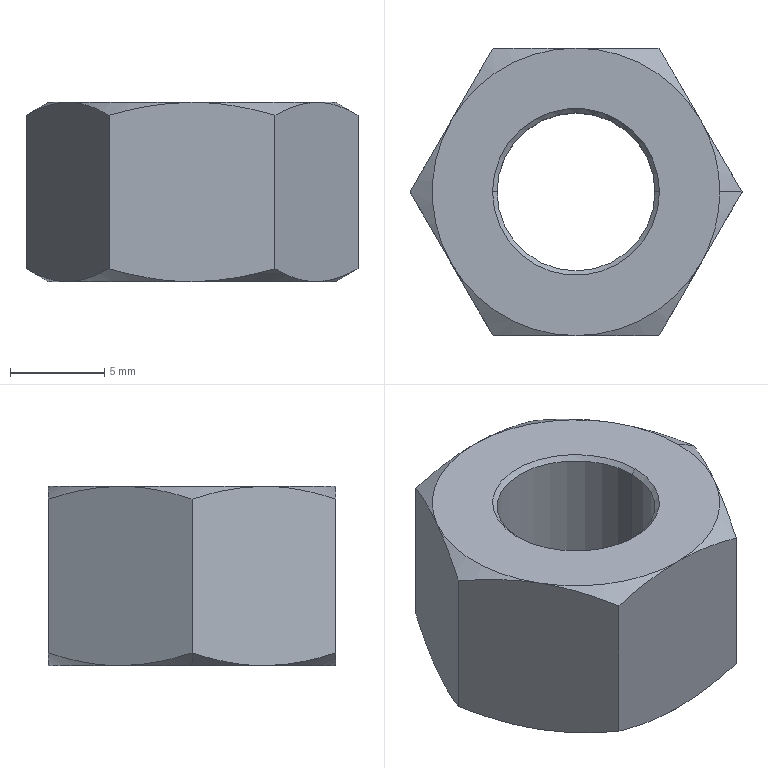Part | SolidWorks | features Cut 2, Chamfer 1, Extrusion 1 | 1 solid | 28 faces | box 17.6 x 15.242 x 9.5 mm | volume 1379 mm3 | cone 18 | plane 8 | cylinder 2 | commonest cylinder face diameters 8.376 x2
STEP:
#1=CARTESIAN_POINT('',(-4.188,0.,9.262));
#2=VERTEX_POINT('',#1);
#3=CARTESIAN_POINT('',(4.188,0.,9.262));
#4=VERTEX_POINT('',#3);
#5=CARTESIAN_POINT('',(0.,0.,9.262));
#6=DIRECTION('',(0.,0.,1.));
#7=DIRECTION('',(-1.,0.,0.));
#8=AXIS2_PLACEMENT_3D('',#5,#6,#7);
#9=CIRCLE('',#8,4.188);
#10=EDGE_CURVE('',#2,#4,#9,.T.);
#11=ORIENTED_EDGE('',*,*,#10,.F.);
#12=CARTESIAN_POINT('',(-4.426,0.,9.5));
#13=VERTEX_POINT('',#12);
#14=CARTESIAN_POINT('',(-4.188,0.,9.262));
#15=DIRECTION('',(-0.7071,0.,0.7071));
#16=VECTOR('',#15,1000.);
#17=LINE('',#14,#16);
#18=EDGE_CURVE('',#2,#13,#17,.T.);
#19=ORIENTED_EDGE('',*,*,#18,.T.);
#20=CARTESIAN_POINT('',(4.426,0.,9.5));
#21=VERTEX_POINT('',#20);
#22=CARTESIAN_POINT('',(0.,0.,9.5));
#23=DIRECTION('',(0.,0.,-1.));
#24=DIRECTION('',(-1.,0.,0.));
#25=AXIS2_PLACEMENT_3D('',#22,#23,#24);
#26=CIRCLE('',#25,4.426);
#27=EDGE_CURVE('',#21,#13,#26,.T.);
#28=ORIENTED_EDGE('',*,*,#27,.F.);
#29=CARTESIAN_POINT('',(4.188,0.,9.262));
#30=DIRECTION('',(0.7071,0.,0.7071));
#31=VECTOR('',#30,1000.);
#32=LINE('',#29,#31);
#33=EDGE_CURVE('',#4,#21,#32,.T.);
#34=ORIENTED_EDGE('',*,*,#33,.F.);
#35=EDGE_LOOP('',(#11,#19,#28,#34));
#36=FACE_OUTER_BOUND('',#35,.T.);
#37=CARTESIAN_POINT('',(0.,0.,9.262));
#38=DIRECTION('',(0.,0.,1.));
#39=DIRECTION('',(1.,0.,0.));
#40=AXIS2_PLACEMENT_3D('',#37,#38,#39);
#41=CONICAL_SURFACE('',#40,4.188,0.7854);
#42=ADVANCED_FACE('',(#36),#41,.F.);
#43=CARTESIAN_POINT('',(4.188,0.,0.2375));
#44=VERTEX_POINT('',#43);
#45=CARTESIAN_POINT('',(-4.188,0.,0.2375));
#46=VERTEX_POINT('',#45);
#47=CARTESIAN_POINT('',(0.,0.,0.2375));
#48=DIRECTION('',(0.,0.,-1.));
#49=DIRECTION('',(-1.,0.,0.));
#50=AXIS2_PLACEMENT_3D('',#47,#48,#49);
#51=CIRCLE('',#50,4.188);
#52=EDGE_CURVE('',#44,#46,#51,.T.);
#53=ORIENTED_EDGE('',*,*,#52,.F.);
#54=CARTESIAN_POINT('',(4.426,0.,0.));
#55=VERTEX_POINT('',#54);
#56=CARTESIAN_POINT('',(4.426,0.,0.));
#57=DIRECTION('',(0.7071,0.,-0.7071));
#58=VECTOR('',#57,1000.);
#59=LINE('',#56,#58);
#60=EDGE_CURVE('',#44,#55,#59,.T.);
#61=ORIENTED_EDGE('',*,*,#60,.T.);
#62=CARTESIAN_POINT('',(-4.426,0.,0.));
#63=VERTEX_POINT('',#62);
#64=CARTESIAN_POINT('',(0.,0.,0.));
#65=DIRECTION('',(0.,0.,1.));
#66=DIRECTION('',(-1.,0.,0.));
#67=AXIS2_PLACEMENT_3D('',#64,#65,#66);
#68=CIRCLE('',#67,4.426);
#69=EDGE_CURVE('',#63,#55,#68,.T.);
#70=ORIENTED_EDGE('',*,*,#69,.F.);
#71=CARTESIAN_POINT('',(-4.426,0.,0.));
#72=DIRECTION('',(-0.7071,0.,-0.7071));
#73=VECTOR('',#72,1000.);
#74=LINE('',#71,#73);
#75=EDGE_CURVE('',#46,#63,#74,.T.);
#76=ORIENTED_EDGE('',*,*,#75,.F.);
#77=EDGE_LOOP('',(#53,#61,#70,#76));
#78=FACE_OUTER_BOUND('',#77,.T.);
#79=CARTESIAN_POINT('',(0.,0.,0.));
#80=DIRECTION('',(0.,0.,-1.));
#81=DIRECTION('',(-1.,0.,0.));
#82=AXIS2_PLACEMENT_3D('',#79,#80,#81);
#83=CONICAL_SURFACE('',#82,4.426,0.7854);
#84=ADVANCED_FACE('',(#78),#83,.F.);
#85=CARTESIAN_POINT('',(6.6,3.811,9.5));
#86=VERTEX_POINT('',#85);
#87=CARTESIAN_POINT('',(7.621,0.,9.5));
#88=VERTEX_POINT('',#87);
#89=CARTESIAN_POINT('',(0.,0.,9.5));
#90=DIRECTION('',(0.,0.,-1.));
#91=DIRECTION('',(-1.,0.,0.));
#92=AXIS2_PLACEMENT_3D('',#89,#90,#91);
#93=CIRCLE('',#92,7.621);
#94=EDGE_CURVE('',#86,#88,#93,.T.);
#95=ORIENTED_EDGE('',*,*,#94,.T.);
#96=CARTESIAN_POINT('',(8.8,0.,8.819));
#97=VERTEX_POINT('',#96);
#98=CARTESIAN_POINT('',(7.621,0.,9.5));
#99=DIRECTION('',(0.866,0.,-0.5));
#100=VECTOR('',#99,1000.);
#101=LINE('',#98,#100);
#102=EDGE_CURVE('',#88,#97,#101,.T.);
#103=ORIENTED_EDGE('',*,*,#102,.T.);
#104=CARTESIAN_POINT('',(8.8,0.,8.819));
#105=CARTESIAN_POINT('',(8.44,0.6233,9.027));
#106=CARTESIAN_POINT('',(8.078,1.251,9.198));
#107=CARTESIAN_POINT('',(7.345,2.52,9.435));
#108=CARTESIAN_POINT('',(6.975,3.161,9.5));
#109=CARTESIAN_POINT('',(6.6,3.811,9.5));
#110=B_SPLINE_CURVE_WITH_KNOTS('',3,(#104,#105,#106,#107,#108,#109),.UNSPECIFIED.,.F.,.F.,(4,2,4),(0.000000238,0.002226,0.004452),.UNSPECIFIED.);
#111=EDGE_CURVE('',#97,#86,#110,.T.);
#112=ORIENTED_EDGE('',*,*,#111,.T.);
#113=EDGE_LOOP('',(#95,#103,#112));
#114=FACE_OUTER_BOUND('',#113,.T.);
#115=CARTESIAN_POINT('',(0.,0.,9.5));
#116=DIRECTION('',(0.,0.,-1.));
#117=DIRECTION('',(1.,0.,0.));
#118=AXIS2_PLACEMENT_3D('',#115,#116,#117);
#119=CONICAL_SURFACE('',#118,7.621,1.047);
#120=ADVANCED_FACE('',(#114),#119,.T.);
#121=CARTESIAN_POINT('',(-7.621,0.,0.));
#122=VERTEX_POINT('',#121);
#123=CARTESIAN_POINT('',(-6.6,3.811,0.));
#124=VERTEX_POINT('',#123);
#125=CARTESIAN_POINT('',(0.,0.,0.));
#126=DIRECTION('',(0.,0.,-1.));
#127=DIRECTION('',(-1.,0.,0.));
#128=AXIS2_PLACEMENT_3D('',#125,#126,#127);
#129=CIRCLE('',#128,7.621);
#130=EDGE_CURVE('',#122,#124,#129,.T.);
#131=ORIENTED_EDGE('',*,*,#130,.F.);
#132=CARTESIAN_POINT('',(-8.8,0.,0.6807));
#133=VERTEX_POINT('',#132);
#134=CARTESIAN_POINT('',(-7.621,0.,0.));
#135=DIRECTION('',(-0.866,0.,0.5));
#136=VECTOR('',#135,1000.);
#137=LINE('',#134,#136);
#138=EDGE_CURVE('',#122,#133,#137,.T.);
#139=ORIENTED_EDGE('',*,*,#138,.T.);
#140=CARTESIAN_POINT('',(-8.8,0.,0.6807));
#141=CARTESIAN_POINT('',(-8.44,0.6233,0.4729));
#142=CARTESIAN_POINT('',(-8.078,1.251,0.3017));
#143=CARTESIAN_POINT('',(-7.345,2.52,0.06487));
#144=CARTESIAN_POINT('',(-6.975,3.161,0.));
#145=CARTESIAN_POINT('',(-6.6,3.811,0.));
#146=B_SPLINE_CURVE_WITH_KNOTS('',3,(#140,#141,#142,#143,#144,#145),.UNSPECIFIED.,.F.,.F.,(4,2,4),(0.000000238,0.002226,0.004452),.UNSPECIFIED.);
#147=EDGE_CURVE('',#133,#124,#146,.T.);
#148=ORIENTED_EDGE('',*,*,#147,.T.);
#149=EDGE_LOOP('',(#131,#139,#148));
#150=FACE_OUTER_BOUND('',#149,.T.);
#151=CARTESIAN_POINT('',(0.,0.,0.));
#152=DIRECTION('',(0.,0.,1.));
#153=DIRECTION('',(-1.,0.,0.));
#154=AXIS2_PLACEMENT_3D('',#151,#152,#153);
#155=CONICAL_SURFACE('',#154,7.621,1.047);
#156=ADVANCED_FACE('',(#150),#155,.T.);
#157=ORIENTED_EDGE('',*,*,#10,.T.);
#158=CARTESIAN_POINT('',(4.188,0.,9.5));
#159=DIRECTION('',(0.,0.,-1.));
#160=VECTOR('',#159,1000.);
#161=LINE('',#158,#160);
#162=EDGE_CURVE('',#4,#44,#161,.T.);
#163=ORIENTED_EDGE('',*,*,#162,.T.);
#164=ORIENTED_EDGE('',*,*,#52,.T.);
#165=CARTESIAN_POINT('',(-4.188,0.,9.5));
#166=DIRECTION('',(0.,0.,-1.));
#167=VECTOR('',#166,1000.);
#168=LINE('',#165,#167);
#169=EDGE_CURVE('',#2,#46,#168,.T.);
#170=ORIENTED_EDGE('',*,*,#169,.F.);
#171=EDGE_LOOP('',(#157,#163,#164,#170));
#172=FACE_OUTER_BOUND('',#171,.T.);
#173=CARTESIAN_POINT('',(0.,0.,9.5));
#174=DIRECTION('',(0.,0.,-1.));
#175=DIRECTION('',(-1.,0.,0.));
#176=AXIS2_PLACEMENT_3D('',#173,#174,#175);
#177=CYLINDRICAL_SURFACE('',#176,4.188);
#178=ADVANCED_FACE('',(#172),#177,.F.);
#179=ORIENTED_EDGE('',*,*,#111,.F.);
#180=CARTESIAN_POINT('',(8.8,0.,0.6807));
#181=VERTEX_POINT('',#180);
#182=CARTESIAN_POINT('',(8.8,0.,9.5));
#183=DIRECTION('',(0.,0.,-1.));
#184=VECTOR('',#183,1000.);
#185=LINE('',#182,#184);
#186=EDGE_CURVE('',#97,#181,#185,.T.);
#187=ORIENTED_EDGE('',*,*,#186,.T.);
#188=CARTESIAN_POINT('',(6.6,3.811,0.));
#189=VERTEX_POINT('',#188);
#190=CARTESIAN_POINT('',(6.6,3.811,0.));
#191=CARTESIAN_POINT('',(6.787,3.487,0.));
#192=CARTESIAN_POINT('',(6.974,3.162,0.01609));
#193=CARTESIAN_POINT('',(7.345,2.52,0.07835));
#194=CARTESIAN_POINT('',(7.53,2.201,0.1245));
#195=CARTESIAN_POINT('',(8.079,1.249,0.3023));
#196=CARTESIAN_POINT('',(8.441,0.6218,0.4734));
#197=CARTESIAN_POINT('',(8.8,0.,0.6807));
#198=B_SPLINE_CURVE_WITH_KNOTS('',3,(#190,#191,#192,#193,#194,#195,#196,#197),.UNSPECIFIED.,.F.,.F.,(4,2,2,4),(0.004452,0.005561,0.00667,0.008888),.UNSPECIFIED.);
#199=EDGE_CURVE('',#189,#181,#198,.T.);
#200=ORIENTED_EDGE('',*,*,#199,.F.);
#201=CARTESIAN_POINT('',(4.4,7.621,0.6807));
#202=VERTEX_POINT('',#201);
#203=CARTESIAN_POINT('',(4.4,7.621,0.6807));
#204=CARTESIAN_POINT('',(4.76,6.998,0.4729));
#205=CARTESIAN_POINT('',(5.122,6.37,0.3017));
#206=CARTESIAN_POINT('',(5.855,5.101,0.06487));
#207=CARTESIAN_POINT('',(6.225,4.46,0.));
#208=CARTESIAN_POINT('',(6.6,3.811,0.));
#209=B_SPLINE_CURVE_WITH_KNOTS('',3,(#203,#204,#205,#206,#207,#208),.UNSPECIFIED.,.F.,.F.,(4,2,4),(0.000000238,0.002226,0.004452),.UNSPECIFIED.);
#210=EDGE_CURVE('',#202,#189,#209,.T.);
#211=ORIENTED_EDGE('',*,*,#210,.F.);
#212=CARTESIAN_POINT('',(4.4,7.621,8.819));
#213=VERTEX_POINT('',#212);
#214=CARTESIAN_POINT('',(4.4,7.621,9.5));
#215=DIRECTION('',(0.,0.,-1.));
#216=VECTOR('',#215,1000.);
#217=LINE('',#214,#216);
#218=EDGE_CURVE('',#213,#202,#217,.T.);
#219=ORIENTED_EDGE('',*,*,#218,.F.);
#220=CARTESIAN_POINT('',(6.6,3.811,9.5));
#221=CARTESIAN_POINT('',(6.413,4.134,9.5));
#222=CARTESIAN_POINT('',(6.226,4.459,9.484));
#223=CARTESIAN_POINT('',(5.855,5.101,9.422));
#224=CARTESIAN_POINT('',(5.67,5.42,9.376));
#225=CARTESIAN_POINT('',(5.121,6.372,9.198));
#226=CARTESIAN_POINT('',(4.759,6.999,9.027));
#227=CARTESIAN_POINT('',(4.4,7.621,8.819));
#228=B_SPLINE_CURVE_WITH_KNOTS('',3,(#220,#221,#222,#223,#224,#225,#226,#227),.UNSPECIFIED.,.F.,.F.,(4,2,2,4),(0.004452,0.005561,0.00667,0.008888),.UNSPECIFIED.);
#229=EDGE_CURVE('',#86,#213,#228,.T.);
#230=ORIENTED_EDGE('',*,*,#229,.F.);
#231=EDGE_LOOP('',(#179,#187,#200,#211,#219,#230));
#232=FACE_OUTER_BOUND('',#231,.T.);
#233=CARTESIAN_POINT('',(8.8,0.,9.5));
#234=DIRECTION('',(-0.866,-0.5,0.));
#235=DIRECTION('',(0.5,-0.866,0.));
#236=AXIS2_PLACEMENT_3D('',#233,#234,#235);
#237=PLANE('',#236);
#238=ADVANCED_FACE('',(#232),#237,.F.);
#239=CARTESIAN_POINT('',(0.,7.621,9.5));
#240=VERTEX_POINT('',#239);
#241=CARTESIAN_POINT('',(4.4,7.621,8.819));
#242=CARTESIAN_POINT('',(3.688,7.621,9.025));
#243=CARTESIAN_POINT('',(2.968,7.621,9.196));
#244=CARTESIAN_POINT('',(1.499,7.621,9.434));
#245=CARTESIAN_POINT('',(0.7447,7.621,9.5));
#246=CARTESIAN_POINT('',(0.,7.621,9.5));
#247=B_SPLINE_CURVE_WITH_KNOTS('',3,(#241,#242,#243,#244,#245,#246),.UNSPECIFIED.,.F.,.F.,(4,2,4),(0.02521,0.02744,0.02967),.UNSPECIFIED.);
#248=EDGE_CURVE('',#213,#240,#247,.T.);
#249=ORIENTED_EDGE('',*,*,#248,.F.);
#250=ORIENTED_EDGE('',*,*,#218,.T.);
#251=CARTESIAN_POINT('',(0.,7.621,0.));
#252=VERTEX_POINT('',#251);
#253=CARTESIAN_POINT('',(0.,7.621,0.));
#254=CARTESIAN_POINT('',(0.7447,7.621,0.));
#255=CARTESIAN_POINT('',(1.499,7.621,0.06582));
#256=CARTESIAN_POINT('',(2.968,7.621,0.3043));
#257=CARTESIAN_POINT('',(3.688,7.621,0.4753));
#258=CARTESIAN_POINT('',(4.4,7.621,0.6807));
#259=B_SPLINE_CURVE_WITH_KNOTS('',3,(#253,#254,#255,#256,#257,#258),.UNSPECIFIED.,.F.,.F.,(4,2,4),(0.01252,0.01475,0.01698),.UNSPECIFIED.);
#260=EDGE_CURVE('',#252,#202,#259,.T.);
#261=ORIENTED_EDGE('',*,*,#260,.F.);
#262=CARTESIAN_POINT('',(-4.4,7.621,0.6807));
#263=VERTEX_POINT('',#262);
#264=CARTESIAN_POINT('',(-4.4,7.621,0.6807));
#265=CARTESIAN_POINT('',(-3.684,7.621,0.4739));
#266=CARTESIAN_POINT('',(-2.951,7.621,0.3008));
#267=CARTESIAN_POINT('',(-1.483,7.621,0.06401));
#268=CARTESIAN_POINT('',(-0.7442,7.621,0.));
#269=CARTESIAN_POINT('',(0.,7.621,0.));
#270=B_SPLINE_CURVE_WITH_KNOTS('',3,(#264,#265,#266,#267,#268,#269),.UNSPECIFIED.,.F.,.F.,(4,2,4),(0.008069,0.0103,0.01252),.UNSPECIFIED.);
#271=EDGE_CURVE('',#263,#252,#270,.T.);
#272=ORIENTED_EDGE('',*,*,#271,.F.);
#273=CARTESIAN_POINT('',(-4.4,7.621,8.819));
#274=VERTEX_POINT('',#273);
#275=CARTESIAN_POINT('',(-4.4,7.621,9.5));
#276=DIRECTION('',(0.,0.,-1.));
#277=VECTOR('',#276,1000.);
#278=LINE('',#275,#277);
#279=EDGE_CURVE('',#274,#263,#278,.T.);
#280=ORIENTED_EDGE('',*,*,#279,.F.);
#281=CARTESIAN_POINT('',(0.,7.621,9.5));
#282=CARTESIAN_POINT('',(-0.7442,7.621,9.5));
#283=CARTESIAN_POINT('',(-1.483,7.621,9.436));
#284=CARTESIAN_POINT('',(-2.951,7.621,9.199));
#285=CARTESIAN_POINT('',(-3.684,7.621,9.026));
#286=CARTESIAN_POINT('',(-4.4,7.621,8.819));
#287=B_SPLINE_CURVE_WITH_KNOTS('',3,(#281,#282,#283,#284,#285,#286),.UNSPECIFIED.,.F.,.F.,(4,2,4),(0.02967,0.0319,0.03412),.UNSPECIFIED.);
#288=EDGE_CURVE('',#240,#274,#287,.T.);
#289=ORIENTED_EDGE('',*,*,#288,.F.);
#290=EDGE_LOOP('',(#249,#250,#261,#272,#280,#289));
#291=FACE_OUTER_BOUND('',#290,.T.);
#292=CARTESIAN_POINT('',(4.4,7.621,9.5));
#293=DIRECTION('',(0.,-1.,0.));
#294=DIRECTION('',(1.,0.,0.));
#295=AXIS2_PLACEMENT_3D('',#292,#293,#294);
#296=PLANE('',#295);
#297=ADVANCED_FACE('',(#291),#296,.F.);
#298=CARTESIAN_POINT('',(-6.6,3.811,9.5));
#299=VERTEX_POINT('',#298);
#300=CARTESIAN_POINT('',(-4.4,7.621,8.819));
#301=CARTESIAN_POINT('',(-4.76,6.998,9.027));
#302=CARTESIAN_POINT('',(-5.122,6.37,9.198));
#303=CARTESIAN_POINT('',(-5.855,5.101,9.435));
#304=CARTESIAN_POINT('',(-6.225,4.46,9.5));
#305=CARTESIAN_POINT('',(-6.6,3.811,9.5));
#306=B_SPLINE_CURVE_WITH_KNOTS('',3,(#300,#301,#302,#303,#304,#305),.UNSPECIFIED.,.F.,.F.,(4,2,4),(0.000000238,0.002226,0.004452),.UNSPECIFIED.);
#307=EDGE_CURVE('',#274,#299,#306,.T.);
#308=ORIENTED_EDGE('',*,*,#307,.F.);
#309=ORIENTED_EDGE('',*,*,#279,.T.);
#310=CARTESIAN_POINT('',(-6.6,3.811,0.));
#311=CARTESIAN_POINT('',(-6.413,4.134,0.));
#312=CARTESIAN_POINT('',(-6.226,4.459,0.01609));
#313=CARTESIAN_POINT('',(-5.855,5.101,0.07835));
#314=CARTESIAN_POINT('',(-5.67,5.42,0.1245));
#315=CARTESIAN_POINT('',(-5.121,6.372,0.3023));
#316=CARTESIAN_POINT('',(-4.759,6.999,0.4734));
#317=CARTESIAN_POINT('',(-4.4,7.621,0.6807));
#318=B_SPLINE_CURVE_WITH_KNOTS('',3,(#310,#311,#312,#313,#314,#315,#316,#317),.UNSPECIFIED.,.F.,.F.,(4,2,2,4),(0.004452,0.005561,0.00667,0.008888),.UNSPECIFIED.);
#319=EDGE_CURVE('',#124,#263,#318,.T.);
#320=ORIENTED_EDGE('',*,*,#319,.F.);
#321=ORIENTED_EDGE('',*,*,#147,.F.);
#322=CARTESIAN_POINT('',(-8.8,0.,8.819));
#323=VERTEX_POINT('',#322);
#324=CARTESIAN_POINT('',(-8.8,0.,9.5));
#325=DIRECTION('',(0.,0.,-1.));
#326=VECTOR('',#325,1000.);
#327=LINE('',#324,#326);
#328=EDGE_CURVE('',#323,#133,#327,.T.);
#329=ORIENTED_EDGE('',*,*,#328,.F.);
#330=CARTESIAN_POINT('',(-6.6,3.811,9.5));
#331=CARTESIAN_POINT('',(-6.787,3.487,9.5));
#332=CARTESIAN_POINT('',(-6.974,3.162,9.484));
#333=CARTESIAN_POINT('',(-7.345,2.52,9.422));
#334=CARTESIAN_POINT('',(-7.53,2.201,9.376));
#335=CARTESIAN_POINT('',(-8.079,1.249,9.198));
#336=CARTESIAN_POINT('',(-8.441,0.6218,9.027));
#337=CARTESIAN_POINT('',(-8.8,0.,8.819));
#338=B_SPLINE_CURVE_WITH_KNOTS('',3,(#330,#331,#332,#333,#334,#335,#336,#337),.UNSPECIFIED.,.F.,.F.,(4,2,2,4),(0.004452,0.005561,0.00667,0.008888),.UNSPECIFIED.);
#339=EDGE_CURVE('',#299,#323,#338,.T.);
#340=ORIENTED_EDGE('',*,*,#339,.F.);
#341=EDGE_LOOP('',(#308,#309,#320,#321,#329,#340));
#342=FACE_OUTER_BOUND('',#341,.T.);
#343=CARTESIAN_POINT('',(-4.4,7.621,9.5));
#344=DIRECTION('',(0.866,-0.5,0.));
#345=DIRECTION('',(0.5,0.866,0.));
#346=AXIS2_PLACEMENT_3D('',#343,#344,#345);
#347=PLANE('',#346);
#348=ADVANCED_FACE('',(#342),#347,.F.);
#349=CARTESIAN_POINT('',(-6.6,-3.811,9.5));
#350=VERTEX_POINT('',#349);
#351=CARTESIAN_POINT('',(-8.8,0.,8.819));
#352=CARTESIAN_POINT('',(-8.44,-0.6233,9.027));
#353=CARTESIAN_POINT('',(-8.078,-1.251,9.198));
#354=CARTESIAN_POINT('',(-7.345,-2.52,9.435));
#355=CARTESIAN_POINT('',(-6.975,-3.161,9.5));
#356=CARTESIAN_POINT('',(-6.6,-3.811,9.5));
#357=B_SPLINE_CURVE_WITH_KNOTS('',3,(#351,#352,#353,#354,#355,#356),.UNSPECIFIED.,.F.,.F.,(4,2,4),(0.000000238,0.002226,0.004452),.UNSPECIFIED.);
#358=EDGE_CURVE('',#323,#350,#357,.T.);
#359=ORIENTED_EDGE('',*,*,#358,.F.);
#360=ORIENTED_EDGE('',*,*,#328,.T.);
#361=CARTESIAN_POINT('',(-6.6,-3.811,0.));
#362=VERTEX_POINT('',#361);
#363=CARTESIAN_POINT('',(-6.6,-3.811,0.));
#364=CARTESIAN_POINT('',(-6.787,-3.487,0.));
#365=CARTESIAN_POINT('',(-6.974,-3.162,0.01609));
#366=CARTESIAN_POINT('',(-7.345,-2.52,0.07835));
#367=CARTESIAN_POINT('',(-7.53,-2.201,0.1245));
#368=CARTESIAN_POINT('',(-8.079,-1.249,0.3023));
#369=CARTESIAN_POINT('',(-8.441,-0.6218,0.4734));
#370=CARTESIAN_POINT('',(-8.8,0.,0.6807));
#371=B_SPLINE_CURVE_WITH_KNOTS('',3,(#363,#364,#365,#366,#367,#368,#369,#370),.UNSPECIFIED.,.F.,.F.,(4,2,2,4),(0.004452,0.005561,0.00667,0.008888),.UNSPECIFIED.);
#372=EDGE_CURVE('',#362,#133,#371,.T.);
#373=ORIENTED_EDGE('',*,*,#372,.F.);
#374=CARTESIAN_POINT('',(-4.4,-7.621,0.6807));
#375=VERTEX_POINT('',#374);
#376=CARTESIAN_POINT('',(-4.4,-7.621,0.6807));
#377=CARTESIAN_POINT('',(-4.76,-6.998,0.4729));
#378=CARTESIAN_POINT('',(-5.122,-6.37,0.3017));
#379=CARTESIAN_POINT('',(-5.855,-5.101,0.06487));
#380=CARTESIAN_POINT('',(-6.225,-4.46,0.));
#381=CARTESIAN_POINT('',(-6.6,-3.811,0.));
#382=B_SPLINE_CURVE_WITH_KNOTS('',3,(#376,#377,#378,#379,#380,#381),.UNSPECIFIED.,.F.,.F.,(4,2,4),(0.000000238,0.002226,0.004452),.UNSPECIFIED.);
#383=EDGE_CURVE('',#375,#362,#382,.T.);
#384=ORIENTED_EDGE('',*,*,#383,.F.);
#385=CARTESIAN_POINT('',(-4.4,-7.621,8.819));
#386=VERTEX_POINT('',#385);
#387=CARTESIAN_POINT('',(-4.4,-7.621,9.5));
#388=DIRECTION('',(0.,0.,-1.));
#389=VECTOR('',#388,1000.);
#390=LINE('',#387,#389);
#391=EDGE_CURVE('',#386,#375,#390,.T.);
#392=ORIENTED_EDGE('',*,*,#391,.F.);
#393=CARTESIAN_POINT('',(-6.6,-3.811,9.5));
#394=CARTESIAN_POINT('',(-6.413,-4.134,9.5));
#395=CARTESIAN_POINT('',(-6.226,-4.459,9.484));
#396=CARTESIAN_POINT('',(-5.855,-5.101,9.422));
#397=CARTESIAN_POINT('',(-5.67,-5.42,9.376));
#398=CARTESIAN_POINT('',(-5.121,-6.372,9.198));
#399=CARTESIAN_POINT('',(-4.759,-6.999,9.027));
#400=CARTESIAN_POINT('',(-4.4,-7.621,8.819));
#401=B_SPLINE_CURVE_WITH_KNOTS('',3,(#393,#394,#395,#396,#397,#398,#399,#400),.UNSPECIFIED.,.F.,.F.,(4,2,2,4),(0.004452,0.005561,0.00667,0.008888),.UNSPECIFIED.);
#402=EDGE_CURVE('',#350,#386,#401,.T.);
#403=ORIENTED_EDGE('',*,*,#402,.F.);
#404=EDGE_LOOP('',(#359,#360,#373,#384,#392,#403));
#405=FACE_OUTER_BOUND('',#404,.T.);
#406=CARTESIAN_POINT('',(-8.8,0.,9.5));
#407=DIRECTION('',(0.866,0.5,0.));
#408=DIRECTION('',(-0.5,0.866,0.));
#409=AXIS2_PLACEMENT_3D('',#406,#407,#408);
#410=PLANE('',#409);
#411=ADVANCED_FACE('',(#405),#410,.F.);
#412=CARTESIAN_POINT('',(0.,-7.621,9.5));
#413=VERTEX_POINT('',#412);
#414=CARTESIAN_POINT('',(-4.4,-7.621,8.819));
#415=CARTESIAN_POINT('',(-3.684,-7.621,9.026));
#416=CARTESIAN_POINT('',(-2.951,-7.621,9.199));
#417=CARTESIAN_POINT('',(-1.483,-7.621,9.436));
#418=CARTESIAN_POINT('',(-0.7442,-7.621,9.5));
#419=CARTESIAN_POINT('',(0.,-7.621,9.5));
#420=B_SPLINE_CURVE_WITH_KNOTS('',3,(#414,#415,#416,#417,#418,#419),.UNSPECIFIED.,.F.,.F.,(4,2,4),(0.008069,0.0103,0.01252),.UNSPECIFIED.);
#421=EDGE_CURVE('',#386,#413,#420,.T.);
#422=ORIENTED_EDGE('',*,*,#421,.F.);
#423=ORIENTED_EDGE('',*,*,#391,.T.);
#424=CARTESIAN_POINT('',(0.,-7.621,0.));
#425=VERTEX_POINT('',#424);
#426=CARTESIAN_POINT('',(0.,-7.621,0.));
#427=CARTESIAN_POINT('',(-0.7442,-7.621,0.));
#428=CARTESIAN_POINT('',(-1.483,-7.621,0.06401));
#429=CARTESIAN_POINT('',(-2.951,-7.621,0.3008));
#430=CARTESIAN_POINT('',(-3.684,-7.621,0.4739));
#431=CARTESIAN_POINT('',(-4.4,-7.621,0.6807));
#432=B_SPLINE_CURVE_WITH_KNOTS('',3,(#426,#427,#428,#429,#430,#431),.UNSPECIFIED.,.F.,.F.,(4,2,4),(0.02967,0.0319,0.03412),.UNSPECIFIED.);
#433=EDGE_CURVE('',#425,#375,#432,.T.);
#434=ORIENTED_EDGE('',*,*,#433,.F.);
#435=CARTESIAN_POINT('',(4.4,-7.621,0.6807));
#436=VERTEX_POINT('',#435);
#437=CARTESIAN_POINT('',(4.4,-7.621,0.6807));
#438=CARTESIAN_POINT('',(3.688,-7.621,0.4753));
#439=CARTESIAN_POINT('',(2.968,-7.621,0.3043));
#440=CARTESIAN_POINT('',(1.499,-7.621,0.06582));
#441=CARTESIAN_POINT('',(0.7447,-7.621,0.));
#442=CARTESIAN_POINT('',(0.,-7.621,0.));
#443=B_SPLINE_CURVE_WITH_KNOTS('',3,(#437,#438,#439,#440,#441,#442),.UNSPECIFIED.,.F.,.F.,(4,2,4),(0.02521,0.02744,0.02967),.UNSPECIFIED.);
#444=EDGE_CURVE('',#436,#425,#443,.T.);
#445=ORIENTED_EDGE('',*,*,#444,.F.);
#446=CARTESIAN_POINT('',(4.4,-7.621,8.819));
#447=VERTEX_POINT('',#446);
#448=CARTESIAN_POINT('',(4.4,-7.621,9.5));
#449=DIRECTION('',(0.,0.,-1.));
#450=VECTOR('',#449,1000.);
#451=LINE('',#448,#450);
#452=EDGE_CURVE('',#447,#436,#451,.T.);
#453=ORIENTED_EDGE('',*,*,#452,.F.);
#454=CARTESIAN_POINT('',(0.,-7.621,9.5));
#455=CARTESIAN_POINT('',(0.7447,-7.621,9.5));
#456=CARTESIAN_POINT('',(1.499,-7.621,9.434));
#457=CARTESIAN_POINT('',(2.968,-7.621,9.196));
#458=CARTESIAN_POINT('',(3.688,-7.621,9.025));
#459=CARTESIAN_POINT('',(4.4,-7.621,8.819));
#460=B_SPLINE_CURVE_WITH_KNOTS('',3,(#454,#455,#456,#457,#458,#459),.UNSPECIFIED.,.F.,.F.,(4,2,4),(0.01252,0.01475,0.01698),.UNSPECIFIED.);
#461=EDGE_CURVE('',#413,#447,#460,.T.);
#462=ORIENTED_EDGE('',*,*,#461,.F.);
#463=EDGE_LOOP('',(#422,#423,#434,#445,#453,#462));
#464=FACE_OUTER_BOUND('',#463,.T.);
#465=CARTESIAN_POINT('',(-4.4,-7.621,9.5));
#466=DIRECTION('',(0.,1.,0.));
#467=DIRECTION('',(0.,0.,1.));
#468=AXIS2_PLACEMENT_3D('',#465,#466,#467);
#469=PLANE('',#468);
#470=ADVANCED_FACE('',(#464),#469,.F.);
#471=CARTESIAN_POINT('',(6.6,-3.811,9.5));
#472=VERTEX_POINT('',#471);
#473=CARTESIAN_POINT('',(4.4,-7.621,8.819));
#474=CARTESIAN_POINT('',(4.76,-6.998,9.027));
#475=CARTESIAN_POINT('',(5.122,-6.37,9.198));
#476=CARTESIAN_POINT('',(5.855,-5.101,9.435));
#477=CARTESIAN_POINT('',(6.225,-4.46,9.5));
#478=CARTESIAN_POINT('',(6.6,-3.811,9.5));
#479=B_SPLINE_CURVE_WITH_KNOTS('',3,(#473,#474,#475,#476,#477,#478),.UNSPECIFIED.,.F.,.F.,(4,2,4),(0.000000238,0.002226,0.004452),.UNSPECIFIED.);
#480=EDGE_CURVE('',#447,#472,#479,.T.);
#481=ORIENTED_EDGE('',*,*,#480,.F.);
#482=ORIENTED_EDGE('',*,*,#452,.T.);
#483=CARTESIAN_POINT('',(6.6,-3.811,0.));
#484=VERTEX_POINT('',#483);
#485=CARTESIAN_POINT('',(6.6,-3.811,0.));
#486=CARTESIAN_POINT('',(6.413,-4.134,0.));
#487=CARTESIAN_POINT('',(6.226,-4.459,0.01609));
#488=CARTESIAN_POINT('',(5.855,-5.101,0.07835));
#489=CARTESIAN_POINT('',(5.67,-5.42,0.1245));
#490=CARTESIAN_POINT('',(5.121,-6.372,0.3023));
#491=CARTESIAN_POINT('',(4.759,-6.999,0.4734));
#492=CARTESIAN_POINT('',(4.4,-7.621,0.6807));
#493=B_SPLINE_CURVE_WITH_KNOTS('',3,(#485,#486,#487,#488,#489,#490,#491,#492),.UNSPECIFIED.,.F.,.F.,(4,2,2,4),(0.004452,0.005561,0.00667,0.008888),.UNSPECIFIED.);
#494=EDGE_CURVE('',#484,#436,#493,.T.);
#495=ORIENTED_EDGE('',*,*,#494,.F.);
#496=CARTESIAN_POINT('',(8.8,0.,0.6807));
#497=CARTESIAN_POINT('',(8.44,-0.6233,0.4729));
#498=CARTESIAN_POINT('',(8.078,-1.251,0.3017));
#499=CARTESIAN_POINT('',(7.345,-2.52,0.06487));
#500=CARTESIAN_POINT('',(6.975,-3.161,0.));
#501=CARTESIAN_POINT('',(6.6,-3.811,0.));
#502=B_SPLINE_CURVE_WITH_KNOTS('',3,(#496,#497,#498,#499,#500,#501),.UNSPECIFIED.,.F.,.F.,(4,2,4),(0.000000238,0.002226,0.004452),.UNSPECIFIED.);
#503=EDGE_CURVE('',#181,#484,#502,.T.);
#504=ORIENTED_EDGE('',*,*,#503,.F.);
#505=ORIENTED_EDGE('',*,*,#186,.F.);
#506=CARTESIAN_POINT('',(6.6,-3.811,9.5));
#507=CARTESIAN_POINT('',(6.787,-3.487,9.5));
#508=CARTESIAN_POINT('',(6.974,-3.162,9.484));
#509=CARTESIAN_POINT('',(7.345,-2.52,9.422));
#510=CARTESIAN_POINT('',(7.53,-2.201,9.376));
#511=CARTESIAN_POINT('',(8.079,-1.249,9.198));
#512=CARTESIAN_POINT('',(8.441,-0.6218,9.027));
#513=CARTESIAN_POINT('',(8.8,0.,8.819));
#514=B_SPLINE_CURVE_WITH_KNOTS('',3,(#506,#507,#508,#509,#510,#511,#512,#513),.UNSPECIFIED.,.F.,.F.,(4,2,2,4),(0.004452,0.005561,0.00667,0.008888),.UNSPECIFIED.);
#515=EDGE_CURVE('',#472,#97,#514,.T.);
#516=ORIENTED_EDGE('',*,*,#515,.F.);
#517=EDGE_LOOP('',(#481,#482,#495,#504,#505,#516));
#518=FACE_OUTER_BOUND('',#517,.T.);
#519=CARTESIAN_POINT('',(4.4,-7.621,9.5));
#520=DIRECTION('',(-0.866,0.5,0.));
#521=DIRECTION('',(-0.5,-0.866,0.));
#522=AXIS2_PLACEMENT_3D('',#519,#520,#521);
#523=PLANE('',#522);
#524=ADVANCED_FACE('',(#518),#523,.F.);
#525=ORIENTED_EDGE('',*,*,#27,.T.);
#526=CARTESIAN_POINT('',(0.,0.,9.5));
#527=DIRECTION('',(0.,0.,-1.));
#528=DIRECTION('',(-1.,0.,0.));
#529=AXIS2_PLACEMENT_3D('',#526,#527,#528);
#530=CIRCLE('',#529,4.426);
#531=EDGE_CURVE('',#13,#21,#530,.T.);
#532=ORIENTED_EDGE('',*,*,#531,.T.);
#533=EDGE_LOOP('',(#525,#532));
#534=FACE_BOUND('',#533,.T.);
#535=CARTESIAN_POINT('',(0.,0.,9.5));
#536=DIRECTION('',(0.,0.,-1.));
#537=DIRECTION('',(-1.,0.,0.));
#538=AXIS2_PLACEMENT_3D('',#535,#536,#537);
#539=CIRCLE('',#538,7.621);
#540=EDGE_CURVE('',#299,#240,#539,.T.);
#541=ORIENTED_EDGE('',*,*,#540,.F.);
#542=CARTESIAN_POINT('',(0.,0.,9.5));
#543=DIRECTION('',(0.,0.,-1.));
#544=DIRECTION('',(-1.,0.,0.));
#545=AXIS2_PLACEMENT_3D('',#542,#543,#544);
#546=CIRCLE('',#545,7.621);
#547=EDGE_CURVE('',#350,#299,#546,.T.);
#548=ORIENTED_EDGE('',*,*,#547,.F.);
#549=CARTESIAN_POINT('',(0.,0.,9.5));
#550=DIRECTION('',(0.,0.,-1.));
#551=DIRECTION('',(-1.,0.,0.));
#552=AXIS2_PLACEMENT_3D('',#549,#550,#551);
#553=CIRCLE('',#552,7.621);
#554=EDGE_CURVE('',#413,#350,#553,.T.);
#555=ORIENTED_EDGE('',*,*,#554,.F.);
#556=CARTESIAN_POINT('',(0.,0.,9.5));
#557=DIRECTION('',(0.,0.,-1.));
#558=DIRECTION('',(-1.,0.,0.));
#559=AXIS2_PLACEMENT_3D('',#556,#557,#558);
#560=CIRCLE('',#559,7.621);
#561=EDGE_CURVE('',#472,#413,#560,.T.);
#562=ORIENTED_EDGE('',*,*,#561,.F.);
#563=CARTESIAN_POINT('',(0.,0.,9.5));
#564=DIRECTION('',(0.,0.,-1.));
#565=DIRECTION('',(-1.,0.,0.));
#566=AXIS2_PLACEMENT_3D('',#563,#564,#565);
#567=CIRCLE('',#566,7.621);
#568=EDGE_CURVE('',#88,#472,#567,.T.);
#569=ORIENTED_EDGE('',*,*,#568,.F.);
#570=ORIENTED_EDGE('',*,*,#94,.F.);
#571=CARTESIAN_POINT('',(0.,0.,9.5));
#572=DIRECTION('',(0.,0.,1.));
#573=DIRECTION('',(1.,0.,0.));
#574=AXIS2_PLACEMENT_3D('',#571,#572,#573);
#575=CIRCLE('',#574,7.621);
#576=EDGE_CURVE('',#86,#240,#575,.T.);
#577=ORIENTED_EDGE('',*,*,#576,.T.);
#578=EDGE_LOOP('',(#541,#548,#555,#562,#569,#570,#577));
#579=FACE_OUTER_BOUND('',#578,.T.);
#580=CARTESIAN_POINT('',(8.8,0.,9.5));
#581=DIRECTION('',(0.,0.,-1.));
#582=DIRECTION('',(-1.,0.,0.));
#583=AXIS2_PLACEMENT_3D('',#580,#581,#582);
#584=PLANE('',#583);
#585=ADVANCED_FACE('',(#534,#579),#584,.F.);
#586=ORIENTED_EDGE('',*,*,#69,.T.);
#587=CARTESIAN_POINT('',(0.,0.,0.));
#588=DIRECTION('',(0.,0.,1.));
#589=DIRECTION('',(-1.,0.,0.));
#590=AXIS2_PLACEMENT_3D('',#587,#588,#589);
#591=CIRCLE('',#590,4.426);
#592=EDGE_CURVE('',#55,#63,#591,.T.);
#593=ORIENTED_EDGE('',*,*,#592,.T.);
#594=EDGE_LOOP('',(#586,#593));
#595=FACE_BOUND('',#594,.T.);
#596=CARTESIAN_POINT('',(0.,0.,0.));
#597=DIRECTION('',(0.,0.,-1.));
#598=DIRECTION('',(-1.,0.,0.));
#599=AXIS2_PLACEMENT_3D('',#596,#597,#598);
#600=CIRCLE('',#599,7.621);
#601=EDGE_CURVE('',#362,#122,#600,.T.);
#602=ORIENTED_EDGE('',*,*,#601,.T.);
#603=ORIENTED_EDGE('',*,*,#130,.T.);
#604=CARTESIAN_POINT('',(0.,0.,0.));
#605=DIRECTION('',(0.,0.,-1.));
#606=DIRECTION('',(-1.,0.,0.));
#607=AXIS2_PLACEMENT_3D('',#604,#605,#606);
#608=CIRCLE('',#607,7.621);
#609=EDGE_CURVE('',#124,#252,#608,.T.);
#610=ORIENTED_EDGE('',*,*,#609,.T.);
#611=CARTESIAN_POINT('',(0.,0.,0.));
#612=DIRECTION('',(0.,0.,-1.));
#613=DIRECTION('',(-1.,0.,0.));
#614=AXIS2_PLACEMENT_3D('',#611,#612,#613);
#615=CIRCLE('',#614,7.621);
#616=EDGE_CURVE('',#252,#189,#615,.T.);
#617=ORIENTED_EDGE('',*,*,#616,.T.);
#618=CARTESIAN_POINT('',(0.,0.,0.));
#619=DIRECTION('',(0.,0.,-1.));
#620=DIRECTION('',(-1.,0.,0.));
#621=AXIS2_PLACEMENT_3D('',#618,#619,#620);
#622=CIRCLE('',#621,7.621);
#623=EDGE_CURVE('',#189,#484,#622,.T.);
#624=ORIENTED_EDGE('',*,*,#623,.T.);
#625=CARTESIAN_POINT('',(0.,0.,0.));
#626=DIRECTION('',(0.,0.,-1.));
#627=DIRECTION('',(-1.,0.,0.));
#628=AXIS2_PLACEMENT_3D('',#625,#626,#627);
#629=CIRCLE('',#628,7.621);
#630=EDGE_CURVE('',#484,#425,#629,.T.);
#631=ORIENTED_EDGE('',*,*,#630,.T.);
#632=CARTESIAN_POINT('',(0.,0.,0.));
#633=DIRECTION('',(0.,0.,-1.));
#634=DIRECTION('',(-1.,0.,0.));
#635=AXIS2_PLACEMENT_3D('',#632,#633,#634);
#636=CIRCLE('',#635,7.621);
#637=EDGE_CURVE('',#425,#362,#636,.T.);
#638=ORIENTED_EDGE('',*,*,#637,.T.);
#639=EDGE_LOOP('',(#602,#603,#610,#617,#624,#631,#638));
#640=FACE_OUTER_BOUND('',#639,.T.);
#641=CARTESIAN_POINT('',(8.8,0.,0.));
#642=DIRECTION('',(0.,0.,-1.));
#643=DIRECTION('',(-1.,0.,0.));
#644=AXIS2_PLACEMENT_3D('',#641,#642,#643);
#645=PLANE('',#644);
#646=ADVANCED_FACE('',(#595,#640),#645,.T.);
#647=ORIENTED_EDGE('',*,*,#162,.F.);
#648=CARTESIAN_POINT('',(0.,0.,9.262));
#649=DIRECTION('',(0.,0.,1.));
#650=DIRECTION('',(-1.,0.,0.));
#651=AXIS2_PLACEMENT_3D('',#648,#649,#650);
#652=CIRCLE('',#651,4.188);
#653=EDGE_CURVE('',#4,#2,#652,.T.);
#654=ORIENTED_EDGE('',*,*,#653,.T.);
#655=ORIENTED_EDGE('',*,*,#169,.T.);
#656=CARTESIAN_POINT('',(0.,0.,0.2375));
#657=DIRECTION('',(0.,0.,-1.));
#658=DIRECTION('',(-1.,0.,0.));
#659=AXIS2_PLACEMENT_3D('',#656,#657,#658);
#660=CIRCLE('',#659,4.188);
#661=EDGE_CURVE('',#46,#44,#660,.T.);
#662=ORIENTED_EDGE('',*,*,#661,.T.);
#663=EDGE_LOOP('',(#647,#654,#655,#662));
#664=FACE_OUTER_BOUND('',#663,.T.);
#665=CARTESIAN_POINT('',(0.,0.,9.5));
#666=DIRECTION('',(0.,0.,-1.));
#667=DIRECTION('',(-1.,0.,0.));
#668=AXIS2_PLACEMENT_3D('',#665,#666,#667);
#669=CYLINDRICAL_SURFACE('',#668,4.188);
#670=ADVANCED_FACE('',(#664),#669,.F.);
#671=ORIENTED_EDGE('',*,*,#444,.T.);
#672=ORIENTED_EDGE('',*,*,#630,.F.);
#673=ORIENTED_EDGE('',*,*,#494,.T.);
#674=EDGE_LOOP('',(#671,#672,#673));
#675=FACE_OUTER_BOUND('',#674,.T.);
#676=CARTESIAN_POINT('',(0.,0.,0.));
#677=DIRECTION('',(0.,0.,1.));
#678=DIRECTION('',(-1.,0.,0.));
#679=AXIS2_PLACEMENT_3D('',#676,#677,#678);
#680=CONICAL_SURFACE('',#679,7.621,1.047);
#681=ADVANCED_FACE('',(#675),#680,.T.);
#682=ORIENTED_EDGE('',*,*,#199,.T.);
#683=ORIENTED_EDGE('',*,*,#503,.T.);
#684=ORIENTED_EDGE('',*,*,#623,.F.);
#685=EDGE_LOOP('',(#682,#683,#684));
#686=FACE_OUTER_BOUND('',#685,.T.);
#687=CARTESIAN_POINT('',(0.,0.,0.));
#688=DIRECTION('',(0.,0.,1.));
#689=DIRECTION('',(-1.,0.,0.));
#690=AXIS2_PLACEMENT_3D('',#687,#688,#689);
#691=CONICAL_SURFACE('',#690,7.621,1.047);
#692=ADVANCED_FACE('',(#686),#691,.T.);
#693=ORIENTED_EDGE('',*,*,#383,.T.);
#694=ORIENTED_EDGE('',*,*,#637,.F.);
#695=ORIENTED_EDGE('',*,*,#433,.T.);
#696=EDGE_LOOP('',(#693,#694,#695));
#697=FACE_OUTER_BOUND('',#696,.T.);
#698=CARTESIAN_POINT('',(0.,0.,0.));
#699=DIRECTION('',(0.,0.,1.));
#700=DIRECTION('',(-1.,0.,0.));
#701=AXIS2_PLACEMENT_3D('',#698,#699,#700);
#702=CONICAL_SURFACE('',#701,7.621,1.047);
#703=ADVANCED_FACE('',(#697),#702,.T.);
#704=ORIENTED_EDGE('',*,*,#138,.F.);
#705=ORIENTED_EDGE('',*,*,#601,.F.);
#706=ORIENTED_EDGE('',*,*,#372,.T.);
#707=EDGE_LOOP('',(#704,#705,#706));
#708=FACE_OUTER_BOUND('',#707,.T.);
#709=CARTESIAN_POINT('',(0.,0.,0.));
#710=DIRECTION('',(0.,0.,1.));
#711=DIRECTION('',(-1.,0.,0.));
#712=AXIS2_PLACEMENT_3D('',#709,#710,#711);
#713=CONICAL_SURFACE('',#712,7.621,1.047);
#714=ADVANCED_FACE('',(#708),#713,.T.);
#715=ORIENTED_EDGE('',*,*,#319,.T.);
#716=ORIENTED_EDGE('',*,*,#271,.T.);
#717=ORIENTED_EDGE('',*,*,#609,.F.);
#718=EDGE_LOOP('',(#715,#716,#717));
#719=FACE_OUTER_BOUND('',#718,.T.);
#720=CARTESIAN_POINT('',(0.,0.,0.));
#721=DIRECTION('',(0.,0.,1.));
#722=DIRECTION('',(-1.,0.,0.));
#723=AXIS2_PLACEMENT_3D('',#720,#721,#722);
#724=CONICAL_SURFACE('',#723,7.621,1.047);
#725=ADVANCED_FACE('',(#719),#724,.T.);
#726=ORIENTED_EDGE('',*,*,#260,.T.);
#727=ORIENTED_EDGE('',*,*,#210,.T.);
#728=ORIENTED_EDGE('',*,*,#616,.F.);
#729=EDGE_LOOP('',(#726,#727,#728));
#730=FACE_OUTER_BOUND('',#729,.T.);
#731=CARTESIAN_POINT('',(0.,0.,0.));
#732=DIRECTION('',(0.,0.,1.));
#733=DIRECTION('',(-1.,0.,0.));
#734=AXIS2_PLACEMENT_3D('',#731,#732,#733);
#735=CONICAL_SURFACE('',#734,7.621,1.047);
#736=ADVANCED_FACE('',(#730),#735,.T.);
#737=ORIENTED_EDGE('',*,*,#339,.T.);
#738=ORIENTED_EDGE('',*,*,#358,.T.);
#739=ORIENTED_EDGE('',*,*,#547,.T.);
#740=EDGE_LOOP('',(#737,#738,#739));
#741=FACE_OUTER_BOUND('',#740,.T.);
#742=CARTESIAN_POINT('',(0.,0.,9.5));
#743=DIRECTION('',(0.,0.,-1.));
#744=DIRECTION('',(1.,0.,0.));
#745=AXIS2_PLACEMENT_3D('',#742,#743,#744);
#746=CONICAL_SURFACE('',#745,7.621,1.047);
#747=ADVANCED_FACE('',(#741),#746,.T.);
#748=ORIENTED_EDGE('',*,*,#402,.T.);
#749=ORIENTED_EDGE('',*,*,#421,.T.);
#750=ORIENTED_EDGE('',*,*,#554,.T.);
#751=EDGE_LOOP('',(#748,#749,#750));
#752=FACE_OUTER_BOUND('',#751,.T.);
#753=CARTESIAN_POINT('',(0.,0.,9.5));
#754=DIRECTION('',(0.,0.,-1.));
#755=DIRECTION('',(1.,0.,0.));
#756=AXIS2_PLACEMENT_3D('',#753,#754,#755);
#757=CONICAL_SURFACE('',#756,7.621,1.047);
#758=ADVANCED_FACE('',(#752),#757,.T.);
#759=ORIENTED_EDGE('',*,*,#461,.T.);
#760=ORIENTED_EDGE('',*,*,#480,.T.);
#761=ORIENTED_EDGE('',*,*,#561,.T.);
#762=EDGE_LOOP('',(#759,#760,#761));
#763=FACE_OUTER_BOUND('',#762,.T.);
#764=CARTESIAN_POINT('',(0.,0.,9.5));
#765=DIRECTION('',(0.,0.,-1.));
#766=DIRECTION('',(1.,0.,0.));
#767=AXIS2_PLACEMENT_3D('',#764,#765,#766);
#768=CONICAL_SURFACE('',#767,7.621,1.047);
#769=ADVANCED_FACE('',(#763),#768,.T.);
#770=ORIENTED_EDGE('',*,*,#102,.F.);
#771=ORIENTED_EDGE('',*,*,#568,.T.);
#772=ORIENTED_EDGE('',*,*,#515,.T.);
#773=EDGE_LOOP('',(#770,#771,#772));
#774=FACE_OUTER_BOUND('',#773,.T.);
#775=CARTESIAN_POINT('',(0.,0.,9.5));
#776=DIRECTION('',(0.,0.,-1.));
#777=DIRECTION('',(1.,0.,0.));
#778=AXIS2_PLACEMENT_3D('',#775,#776,#777);
#779=CONICAL_SURFACE('',#778,7.621,1.047);
#780=ADVANCED_FACE('',(#774),#779,.T.);
#781=ORIENTED_EDGE('',*,*,#229,.T.);
#782=ORIENTED_EDGE('',*,*,#248,.T.);
#783=ORIENTED_EDGE('',*,*,#576,.F.);
#784=EDGE_LOOP('',(#781,#782,#783));
#785=FACE_OUTER_BOUND('',#784,.T.);
#786=CARTESIAN_POINT('',(0.,0.,9.5));
#787=DIRECTION('',(0.,0.,-1.));
#788=DIRECTION('',(1.,0.,0.));
#789=AXIS2_PLACEMENT_3D('',#786,#787,#788);
#790=CONICAL_SURFACE('',#789,7.621,1.047);
#791=ADVANCED_FACE('',(#785),#790,.T.);
#792=ORIENTED_EDGE('',*,*,#288,.T.);
#793=ORIENTED_EDGE('',*,*,#307,.T.);
#794=ORIENTED_EDGE('',*,*,#540,.T.);
#795=EDGE_LOOP('',(#792,#793,#794));
#796=FACE_OUTER_BOUND('',#795,.T.);
#797=CARTESIAN_POINT('',(0.,0.,9.5));
#798=DIRECTION('',(0.,0.,-1.));
#799=DIRECTION('',(1.,0.,0.));
#800=AXIS2_PLACEMENT_3D('',#797,#798,#799);
#801=CONICAL_SURFACE('',#800,7.621,1.047);
#802=ADVANCED_FACE('',(#796),#801,.T.);
#803=ORIENTED_EDGE('',*,*,#60,.F.);
#804=ORIENTED_EDGE('',*,*,#661,.F.);
#805=ORIENTED_EDGE('',*,*,#75,.T.);
#806=ORIENTED_EDGE('',*,*,#592,.F.);
#807=EDGE_LOOP('',(#803,#804,#805,#806));
#808=FACE_OUTER_BOUND('',#807,.T.);
#809=CARTESIAN_POINT('',(0.,0.,0.));
#810=DIRECTION('',(0.,0.,-1.));
#811=DIRECTION('',(-1.,0.,0.));
#812=AXIS2_PLACEMENT_3D('',#809,#810,#811);
#813=CONICAL_SURFACE('',#812,4.426,0.7854);
#814=ADVANCED_FACE('',(#808),#813,.F.);
#815=ORIENTED_EDGE('',*,*,#18,.F.);
#816=ORIENTED_EDGE('',*,*,#653,.F.);
#817=ORIENTED_EDGE('',*,*,#33,.T.);
#818=ORIENTED_EDGE('',*,*,#531,.F.);
#819=EDGE_LOOP('',(#815,#816,#817,#818));
#820=FACE_OUTER_BOUND('',#819,.T.);
#821=CARTESIAN_POINT('',(0.,0.,9.262));
#822=DIRECTION('',(0.,0.,1.));
#823=DIRECTION('',(1.,0.,0.));
#824=AXIS2_PLACEMENT_3D('',#821,#822,#823);
#825=CONICAL_SURFACE('',#824,4.188,0.7854);
#826=ADVANCED_FACE('',(#820),#825,.F.);
#827=CLOSED_SHELL('',(#42,#84,#120,#156,#178,#238,#297,#348,#411,#470,#524,#585,#646,#670,#681,#692,#703,#714,#725,#736,#747,#758,#769,#780,#791,#802,#814,#826));
#828=MANIFOLD_SOLID_BREP('',#827);
#829=CARTESIAN_POINT('',(0.,0.,0.));
#830=DIRECTION('',(0.,0.,1.));
#831=DIRECTION('',(1.,0.,0.));
#832=AXIS2_PLACEMENT_3D('',#829,#830,#831);
#833=(LENGTH_UNIT()NAMED_UNIT(*)SI_UNIT(.MILLI.,.METRE.));
#834=UNCERTAINTY_MEASURE_WITH_UNIT(LENGTH_MEASURE(0.00001),#833,'','');
#835=(NAMED_UNIT(*)PLANE_ANGLE_UNIT()SI_UNIT($,.RADIAN.));
#836=(NAMED_UNIT(*)SI_UNIT($,.STERADIAN.)SOLID_ANGLE_UNIT());
#837=(GEOMETRIC_REPRESENTATION_CONTEXT(3)GLOBAL_UNCERTAINTY_ASSIGNED_CONTEXT((#834))GLOBAL_UNIT_ASSIGNED_CONTEXT((#833,#835,#836))REPRESENTATION_CONTEXT('',''));
#838=ADVANCED_BREP_SHAPE_REPRESENTATION('',(#828,#832),#837);